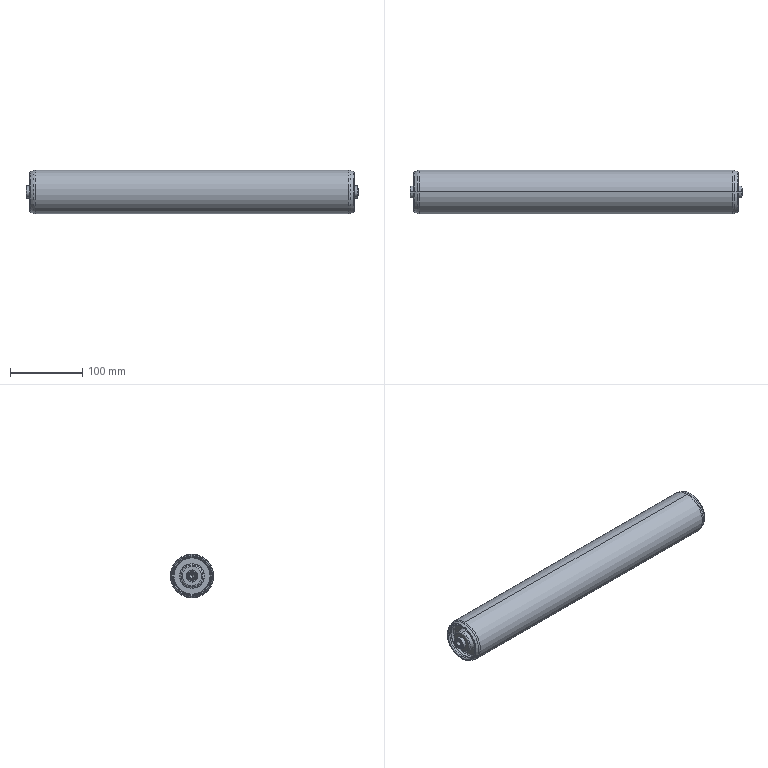Part | SolidWorks | features BaseBody 1, RefAxis 1 | 1 solid | 114 faces | box 459 x 60 x 60 mm | volume 236387 mm3 | spline 48 | cone 28 | cylinder 26 | plane 12 | commonest cylinder face diameters 6.8 x4 16.6 x4 28 x4 30.6 x4 53.6 x4 12 x2